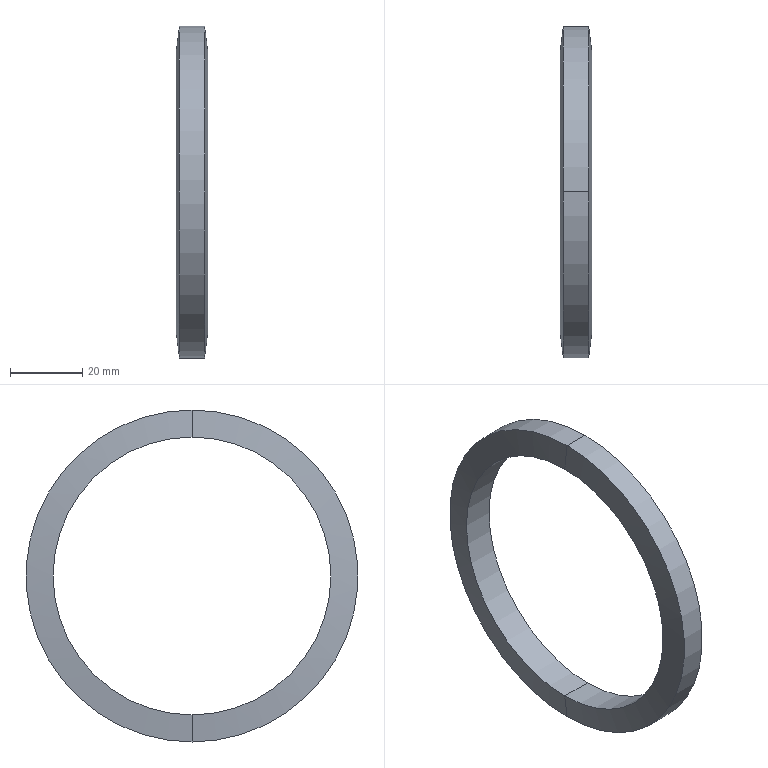Part | SolidWorks | features Sweep 1 | 1 solid | 8 faces | box 8.842 x 92 x 92 mm | volume 15716 mm3 | cone 4 | cylinder 4 | commonest cylinder face diameters 77 x2 92 x2
STEP:
#1=CARTESIAN_POINT('',(4.421,-46.,-38.5));
#2=VERTEX_POINT('',#1);
#3=CARTESIAN_POINT('',(4.421,-46.,38.5));
#4=VERTEX_POINT('',#3);
#5=CARTESIAN_POINT('',(4.421,-46.,0.));
#6=DIRECTION('',(1.,0.,0.));
#7=DIRECTION('',(0.,1.,0.));
#8=AXIS2_PLACEMENT_3D('',#5,#6,#7);
#9=CIRCLE('',#8,38.5);
#10=EDGE_CURVE('',#2,#4,#9,.T.);
#11=ORIENTED_EDGE('',*,*,#10,.F.);
#12=CARTESIAN_POINT('',(3.5,-46.,-46.));
#13=VERTEX_POINT('',#12);
#14=CARTESIAN_POINT('',(4.421,-46.,-38.5));
#15=DIRECTION('',(-0.1219,0.,-0.9925));
#16=VECTOR('',#15,1000.);
#17=LINE('',#14,#16);
#18=EDGE_CURVE('',#2,#13,#17,.T.);
#19=ORIENTED_EDGE('',*,*,#18,.T.);
#20=CARTESIAN_POINT('',(3.5,-46.,46.));
#21=VERTEX_POINT('',#20);
#22=CARTESIAN_POINT('',(3.5,-46.,0.));
#23=DIRECTION('',(1.,0.,0.));
#24=DIRECTION('',(0.,1.,0.));
#25=AXIS2_PLACEMENT_3D('',#22,#23,#24);
#26=CIRCLE('',#25,46.);
#27=EDGE_CURVE('',#13,#21,#26,.T.);
#28=ORIENTED_EDGE('',*,*,#27,.T.);
#29=CARTESIAN_POINT('',(4.421,-46.,38.5));
#30=DIRECTION('',(-0.1219,0.,0.9925));
#31=VECTOR('',#30,1000.);
#32=LINE('',#29,#31);
#33=EDGE_CURVE('',#4,#21,#32,.T.);
#34=ORIENTED_EDGE('',*,*,#33,.F.);
#35=EDGE_LOOP('',(#11,#19,#28,#34));
#36=FACE_OUTER_BOUND('',#35,.T.);
#37=CARTESIAN_POINT('',(4.421,-46.,0.));
#38=DIRECTION('',(-1.,0.,0.));
#39=DIRECTION('',(0.,0.,1.));
#40=AXIS2_PLACEMENT_3D('',#37,#38,#39);
#41=CONICAL_SURFACE('',#40,38.5,1.449);
#42=ADVANCED_FACE('',(#36),#41,.T.);
#43=CARTESIAN_POINT('',(-3.5,-46.,-46.));
#44=VERTEX_POINT('',#43);
#45=CARTESIAN_POINT('',(-3.5,-46.,46.));
#46=VERTEX_POINT('',#45);
#47=CARTESIAN_POINT('',(-3.5,-46.,0.));
#48=DIRECTION('',(1.,0.,0.));
#49=DIRECTION('',(0.,1.,0.));
#50=AXIS2_PLACEMENT_3D('',#47,#48,#49);
#51=CIRCLE('',#50,46.);
#52=EDGE_CURVE('',#44,#46,#51,.T.);
#53=ORIENTED_EDGE('',*,*,#52,.T.);
#54=CARTESIAN_POINT('',(0.,-46.,46.));
#55=DIRECTION('',(1.,0.,0.));
#56=VECTOR('',#55,1000.);
#57=LINE('',#54,#56);
#58=EDGE_CURVE('',#46,#21,#57,.T.);
#59=ORIENTED_EDGE('',*,*,#58,.T.);
#60=ORIENTED_EDGE('',*,*,#27,.F.);
#61=CARTESIAN_POINT('',(0.,-46.,-46.));
#62=DIRECTION('',(1.,0.,0.));
#63=VECTOR('',#62,1000.);
#64=LINE('',#61,#63);
#65=EDGE_CURVE('',#44,#13,#64,.T.);
#66=ORIENTED_EDGE('',*,*,#65,.F.);
#67=EDGE_LOOP('',(#53,#59,#60,#66));
#68=FACE_OUTER_BOUND('',#67,.T.);
#69=CARTESIAN_POINT('',(0.,-46.,0.));
#70=DIRECTION('',(1.,0.,0.));
#71=DIRECTION('',(0.,0.,-1.));
#72=AXIS2_PLACEMENT_3D('',#69,#70,#71);
#73=CYLINDRICAL_SURFACE('',#72,46.);
#74=ADVANCED_FACE('',(#68),#73,.T.);
#75=CARTESIAN_POINT('',(-4.421,-46.,-38.5));
#76=VERTEX_POINT('',#75);
#77=CARTESIAN_POINT('',(-4.421,-46.,38.5));
#78=VERTEX_POINT('',#77);
#79=CARTESIAN_POINT('',(-4.421,-46.,0.));
#80=DIRECTION('',(1.,0.,0.));
#81=DIRECTION('',(0.,1.,0.));
#82=AXIS2_PLACEMENT_3D('',#79,#80,#81);
#83=CIRCLE('',#82,38.5);
#84=EDGE_CURVE('',#76,#78,#83,.T.);
#85=ORIENTED_EDGE('',*,*,#84,.T.);
#86=CARTESIAN_POINT('',(-3.5,-46.,46.));
#87=DIRECTION('',(0.1219,0.,0.9925));
#88=VECTOR('',#87,1000.);
#89=LINE('',#86,#88);
#90=EDGE_CURVE('',#78,#46,#89,.T.);
#91=ORIENTED_EDGE('',*,*,#90,.T.);
#92=ORIENTED_EDGE('',*,*,#52,.F.);
#93=CARTESIAN_POINT('',(-3.5,-46.,-46.));
#94=DIRECTION('',(0.1219,0.,-0.9925));
#95=VECTOR('',#94,1000.);
#96=LINE('',#93,#95);
#97=EDGE_CURVE('',#76,#44,#96,.T.);
#98=ORIENTED_EDGE('',*,*,#97,.F.);
#99=EDGE_LOOP('',(#85,#91,#92,#98));
#100=FACE_OUTER_BOUND('',#99,.T.);
#101=CARTESIAN_POINT('',(-3.5,-46.,0.));
#102=DIRECTION('',(1.,0.,0.));
#103=DIRECTION('',(0.,0.,-1.));
#104=AXIS2_PLACEMENT_3D('',#101,#102,#103);
#105=CONICAL_SURFACE('',#104,46.,1.449);
#106=ADVANCED_FACE('',(#100),#105,.T.);
#107=CARTESIAN_POINT('',(-4.421,-46.,0.));
#108=DIRECTION('',(1.,0.,0.));
#109=DIRECTION('',(0.,1.,0.));
#110=AXIS2_PLACEMENT_3D('',#107,#108,#109);
#111=CIRCLE('',#110,38.5);
#112=EDGE_CURVE('',#78,#76,#111,.T.);
#113=ORIENTED_EDGE('',*,*,#112,.F.);
#114=CARTESIAN_POINT('',(0.,-46.,38.5));
#115=DIRECTION('',(1.,0.,0.));
#116=VECTOR('',#115,1000.);
#117=LINE('',#114,#116);
#118=EDGE_CURVE('',#78,#4,#117,.T.);
#119=ORIENTED_EDGE('',*,*,#118,.T.);
#120=CARTESIAN_POINT('',(4.421,-46.,0.));
#121=DIRECTION('',(1.,0.,0.));
#122=DIRECTION('',(0.,1.,0.));
#123=AXIS2_PLACEMENT_3D('',#120,#121,#122);
#124=CIRCLE('',#123,38.5);
#125=EDGE_CURVE('',#4,#2,#124,.T.);
#126=ORIENTED_EDGE('',*,*,#125,.T.);
#127=CARTESIAN_POINT('',(0.,-46.,-38.5));
#128=DIRECTION('',(1.,0.,0.));
#129=VECTOR('',#128,1000.);
#130=LINE('',#127,#129);
#131=EDGE_CURVE('',#76,#2,#130,.T.);
#132=ORIENTED_EDGE('',*,*,#131,.F.);
#133=EDGE_LOOP('',(#113,#119,#126,#132));
#134=FACE_OUTER_BOUND('',#133,.T.);
#135=CARTESIAN_POINT('',(0.,-46.,0.));
#136=DIRECTION('',(1.,0.,0.));
#137=DIRECTION('',(0.,0.,-1.));
#138=AXIS2_PLACEMENT_3D('',#135,#136,#137);
#139=CYLINDRICAL_SURFACE('',#138,38.5);
#140=ADVANCED_FACE('',(#134),#139,.F.);
#141=ORIENTED_EDGE('',*,*,#118,.F.);
#142=ORIENTED_EDGE('',*,*,#84,.F.);
#143=ORIENTED_EDGE('',*,*,#131,.T.);
#144=ORIENTED_EDGE('',*,*,#10,.T.);
#145=EDGE_LOOP('',(#141,#142,#143,#144));
#146=FACE_OUTER_BOUND('',#145,.T.);
#147=CARTESIAN_POINT('',(0.,-46.,0.));
#148=DIRECTION('',(1.,0.,0.));
#149=DIRECTION('',(0.,0.,-1.));
#150=AXIS2_PLACEMENT_3D('',#147,#148,#149);
#151=CYLINDRICAL_SURFACE('',#150,38.5);
#152=ADVANCED_FACE('',(#146),#151,.F.);
#153=ORIENTED_EDGE('',*,*,#90,.F.);
#154=ORIENTED_EDGE('',*,*,#112,.T.);
#155=ORIENTED_EDGE('',*,*,#97,.T.);
#156=CARTESIAN_POINT('',(-3.5,-46.,0.));
#157=DIRECTION('',(1.,0.,0.));
#158=DIRECTION('',(0.,1.,0.));
#159=AXIS2_PLACEMENT_3D('',#156,#157,#158);
#160=CIRCLE('',#159,46.);
#161=EDGE_CURVE('',#46,#44,#160,.T.);
#162=ORIENTED_EDGE('',*,*,#161,.F.);
#163=EDGE_LOOP('',(#153,#154,#155,#162));
#164=FACE_OUTER_BOUND('',#163,.T.);
#165=CARTESIAN_POINT('',(-3.5,-46.,0.));
#166=DIRECTION('',(1.,0.,0.));
#167=DIRECTION('',(0.,0.,-1.));
#168=AXIS2_PLACEMENT_3D('',#165,#166,#167);
#169=CONICAL_SURFACE('',#168,46.,1.449);
#170=ADVANCED_FACE('',(#164),#169,.T.);
#171=ORIENTED_EDGE('',*,*,#58,.F.);
#172=ORIENTED_EDGE('',*,*,#161,.T.);
#173=ORIENTED_EDGE('',*,*,#65,.T.);
#174=CARTESIAN_POINT('',(3.5,-46.,0.));
#175=DIRECTION('',(1.,0.,0.));
#176=DIRECTION('',(0.,1.,0.));
#177=AXIS2_PLACEMENT_3D('',#174,#175,#176);
#178=CIRCLE('',#177,46.);
#179=EDGE_CURVE('',#21,#13,#178,.T.);
#180=ORIENTED_EDGE('',*,*,#179,.F.);
#181=EDGE_LOOP('',(#171,#172,#173,#180));
#182=FACE_OUTER_BOUND('',#181,.T.);
#183=CARTESIAN_POINT('',(0.,-46.,0.));
#184=DIRECTION('',(1.,0.,0.));
#185=DIRECTION('',(0.,0.,-1.));
#186=AXIS2_PLACEMENT_3D('',#183,#184,#185);
#187=CYLINDRICAL_SURFACE('',#186,46.);
#188=ADVANCED_FACE('',(#182),#187,.T.);
#189=ORIENTED_EDGE('',*,*,#18,.F.);
#190=ORIENTED_EDGE('',*,*,#125,.F.);
#191=ORIENTED_EDGE('',*,*,#33,.T.);
#192=ORIENTED_EDGE('',*,*,#179,.T.);
#193=EDGE_LOOP('',(#189,#190,#191,#192));
#194=FACE_OUTER_BOUND('',#193,.T.);
#195=CARTESIAN_POINT('',(4.421,-46.,0.));
#196=DIRECTION('',(-1.,0.,0.));
#197=DIRECTION('',(0.,0.,1.));
#198=AXIS2_PLACEMENT_3D('',#195,#196,#197);
#199=CONICAL_SURFACE('',#198,38.5,1.449);
#200=ADVANCED_FACE('',(#194),#199,.T.);
#201=CLOSED_SHELL('',(#42,#74,#106,#140,#152,#170,#188,#200));
#202=MANIFOLD_SOLID_BREP('',#201);
#203=CARTESIAN_POINT('',(0.,0.,0.));
#204=DIRECTION('',(0.,0.,1.));
#205=DIRECTION('',(1.,0.,0.));
#206=AXIS2_PLACEMENT_3D('',#203,#204,#205);
#207=(LENGTH_UNIT()NAMED_UNIT(*)SI_UNIT(.MILLI.,.METRE.));
#208=UNCERTAINTY_MEASURE_WITH_UNIT(LENGTH_MEASURE(0.00001),#207,'','');
#209=(NAMED_UNIT(*)PLANE_ANGLE_UNIT()SI_UNIT($,.RADIAN.));
#210=(NAMED_UNIT(*)SI_UNIT($,.STERADIAN.)SOLID_ANGLE_UNIT());
#211=(GEOMETRIC_REPRESENTATION_CONTEXT(3)GLOBAL_UNCERTAINTY_ASSIGNED_CONTEXT((#208))GLOBAL_UNIT_ASSIGNED_CONTEXT((#207,#209,#210))REPRESENTATION_CONTEXT('',''));
#212=ADVANCED_BREP_SHAPE_REPRESENTATION('',(#202,#206),#211);